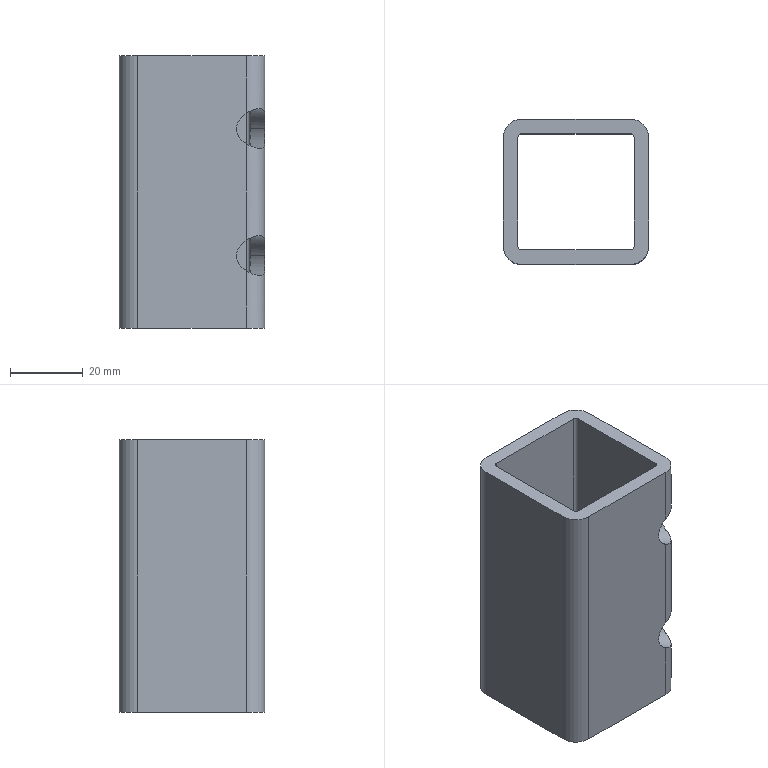Part | SolidWorks | features Extrusion 1, ICE 1 | 1 solid | 26 faces | box 40 x 40 x 75 mm | volume 40690 mm3 | cylinder 16 | plane 10 | commonest cylinder face diameters 2 x6 10 x6 11 x4
STEP:
#1=CARTESIAN_POINT('',(20.,-15.,15.787));
#2=VERTEX_POINT('',#1);
#3=CARTESIAN_POINT('',(20.,-12.222,20.));
#4=VERTEX_POINT('',#3);
#5=CARTESIAN_POINT('',(20.,-15.,15.787));
#6=CARTESIAN_POINT('',(20.,-13.21,16.849));
#7=CARTESIAN_POINT('',(20.,-12.222,18.347));
#8=CARTESIAN_POINT('',(20.,-12.222,20.));
#9=(BOUNDED_CURVE()B_SPLINE_CURVE(3,(#5,#6,#7,#8),.UNSPECIFIED.,.F.,.F.)B_SPLINE_CURVE_WITH_KNOTS((4,4),(5.411,6.283),.UNSPECIFIED.)CURVE()GEOMETRIC_REPRESENTATION_ITEM()RATIONAL_B_SPLINE_CURVE((1.,0.9375,0.9375,1.))REPRESENTATION_ITEM(''));
#10=EDGE_CURVE('',#2,#4,#9,.T.);
#11=ORIENTED_EDGE('',*,*,#10,.T.);
#12=CARTESIAN_POINT('',(16.,-8.222,20.));
#13=VERTEX_POINT('',#12);
#14=CARTESIAN_POINT('',(35.709,-27.931,20.));
#15=DIRECTION('',(-0.7071,0.7071,0.));
#16=VECTOR('',#15,1000.);
#17=LINE('',#14,#16);
#18=EDGE_CURVE('',#4,#13,#17,.T.);
#19=ORIENTED_EDGE('',*,*,#18,.T.);
#20=CARTESIAN_POINT('',(16.,-15.,14.546));
#21=VERTEX_POINT('',#20);
#22=CARTESIAN_POINT('',(16.,-15.,14.546));
#23=CARTESIAN_POINT('',(16.,-10.931,14.919));
#24=CARTESIAN_POINT('',(16.,-8.222,17.098));
#25=CARTESIAN_POINT('',(16.,-8.222,20.));
#26=(BOUNDED_CURVE()B_SPLINE_CURVE(3,(#22,#23,#24,#25),.UNSPECIFIED.,.F.,.F.)B_SPLINE_CURVE_WITH_KNOTS((4,4),(4.841,6.283),.UNSPECIFIED.)CURVE()GEOMETRIC_REPRESENTATION_ITEM()RATIONAL_B_SPLINE_CURVE((1.,0.8341,0.8341,1.))REPRESENTATION_ITEM(''));
#27=EDGE_CURVE('',#21,#13,#26,.T.);
#28=ORIENTED_EDGE('',*,*,#27,.F.);
#29=CARTESIAN_POINT('',(15.,-16.,14.546));
#30=VERTEX_POINT('',#29);
#31=CARTESIAN_POINT('',(16.,-15.,14.546));
#32=CARTESIAN_POINT('',(16.,-15.132,14.534));
#33=CARTESIAN_POINT('',(15.974,-15.261,14.522));
#34=CARTESIAN_POINT('',(15.874,-15.503,14.505));
#35=CARTESIAN_POINT('',(15.8,-15.614,14.5));
#36=CARTESIAN_POINT('',(15.615,-15.799,14.5));
#37=CARTESIAN_POINT('',(15.503,-15.874,14.505));
#38=CARTESIAN_POINT('',(15.263,-15.974,14.522));
#39=CARTESIAN_POINT('',(15.132,-16.,14.534));
#40=CARTESIAN_POINT('',(15.,-16.,14.546));
#41=B_SPLINE_CURVE_WITH_KNOTS('',3,(#31,#32,#33,#34,#35,#36,#37,#38,#39,#40),.UNSPECIFIED.,.F.,.F.,(4,2,2,2,4),(0.,0.0003914,0.0007827,0.001174,0.001565),.UNSPECIFIED.);
#42=EDGE_CURVE('',#21,#30,#41,.T.);
#43=ORIENTED_EDGE('',*,*,#42,.T.);
#44=CARTESIAN_POINT('',(8.222,-16.,20.));
#45=VERTEX_POINT('',#44);
#46=CARTESIAN_POINT('',(15.,-16.,14.546));
#47=CARTESIAN_POINT('',(10.931,-16.,14.919));
#48=CARTESIAN_POINT('',(8.222,-16.,17.098));
#49=CARTESIAN_POINT('',(8.222,-16.,20.));
#50=(BOUNDED_CURVE()B_SPLINE_CURVE(3,(#46,#47,#48,#49),.UNSPECIFIED.,.F.,.F.)B_SPLINE_CURVE_WITH_KNOTS((4,4),(4.841,6.283),.UNSPECIFIED.)CURVE()GEOMETRIC_REPRESENTATION_ITEM()RATIONAL_B_SPLINE_CURVE((1.,0.8341,0.8341,1.))REPRESENTATION_ITEM(''));
#51=EDGE_CURVE('',#30,#45,#50,.T.);
#52=ORIENTED_EDGE('',*,*,#51,.T.);
#53=CARTESIAN_POINT('',(12.222,-20.,20.));
#54=VERTEX_POINT('',#53);
#55=CARTESIAN_POINT('',(27.931,-35.709,20.));
#56=DIRECTION('',(-0.7071,0.7071,0.));
#57=VECTOR('',#56,1000.);
#58=LINE('',#55,#57);
#59=EDGE_CURVE('',#54,#45,#58,.T.);
#60=ORIENTED_EDGE('',*,*,#59,.F.);
#61=CARTESIAN_POINT('',(15.,-20.,15.787));
#62=VERTEX_POINT('',#61);
#63=CARTESIAN_POINT('',(15.,-20.,15.787));
#64=CARTESIAN_POINT('',(13.21,-20.,16.849));
#65=CARTESIAN_POINT('',(12.222,-20.,18.347));
#66=CARTESIAN_POINT('',(12.222,-20.,20.));
#67=(BOUNDED_CURVE()B_SPLINE_CURVE(3,(#63,#64,#65,#66),.UNSPECIFIED.,.F.,.F.)B_SPLINE_CURVE_WITH_KNOTS((4,4),(5.411,6.283),.UNSPECIFIED.)CURVE()GEOMETRIC_REPRESENTATION_ITEM()RATIONAL_B_SPLINE_CURVE((1.,0.9375,0.9375,1.))REPRESENTATION_ITEM(''));
#68=EDGE_CURVE('',#62,#54,#67,.T.);
#69=ORIENTED_EDGE('',*,*,#68,.F.);
#70=CARTESIAN_POINT('',(20.,-15.,15.787));
#71=CARTESIAN_POINT('',(20.,-15.301,15.608));
#72=CARTESIAN_POINT('',(19.973,-15.604,15.44));
#73=CARTESIAN_POINT('',(19.888,-16.063,15.209));
#74=CARTESIAN_POINT('',(19.852,-16.216,15.136));
#75=CARTESIAN_POINT('',(19.764,-16.525,14.997));
#76=CARTESIAN_POINT('',(19.712,-16.68,14.932));
#77=CARTESIAN_POINT('',(19.532,-17.138,14.757));
#78=CARTESIAN_POINT('',(19.38,-17.436,14.664));
#79=CARTESIAN_POINT('',(19.003,-18.016,14.534));
#80=CARTESIAN_POINT('',(18.786,-18.284,14.501));
#81=CARTESIAN_POINT('',(18.419,-18.653,14.5));
#82=CARTESIAN_POINT('',(18.288,-18.771,14.508));
#83=CARTESIAN_POINT('',(18.017,-18.991,14.54));
#84=CARTESIAN_POINT('',(17.878,-19.092,14.565));
#85=CARTESIAN_POINT('',(17.449,-19.373,14.66));
#86=CARTESIAN_POINT('',(17.144,-19.529,14.755));
#87=CARTESIAN_POINT('',(16.534,-19.77,14.988));
#88=CARTESIAN_POINT('',(16.224,-19.858,15.128));
#89=CARTESIAN_POINT('',(15.606,-19.973,15.438));
#90=CARTESIAN_POINT('',(15.302,-20.,15.608));
#91=CARTESIAN_POINT('',(15.,-20.,15.787));
#92=B_SPLINE_CURVE_WITH_KNOTS('',3,(#70,#71,#72,#73,#74,#75,#76,#77,#78,#79,#80,#81,#82,#83,#84,#85,#86,#87,#88,#89,#90,#91),.UNSPECIFIED.,.F.,.F.,(4,2,2,2,2,2,2,2,2,2,4),(0.,0.00104,0.00156,0.00208,0.00312,0.00416,0.00468,0.0052,0.00624,0.00728,0.00832),.UNSPECIFIED.);
#93=EDGE_CURVE('',#2,#62,#92,.T.);
#94=ORIENTED_EDGE('',*,*,#93,.F.);
#95=EDGE_LOOP('',(#11,#19,#28,#43,#52,#60,#69,#94));
#96=FACE_OUTER_BOUND('',#95,.T.);
#97=CARTESIAN_POINT('',(31.82,-31.82,20.));
#98=DIRECTION('',(-0.7071,0.7071,0.));
#99=DIRECTION('',(-0.7071,-0.7071,0.));
#100=AXIS2_PLACEMENT_3D('',#97,#98,#99);
#101=CYLINDRICAL_SURFACE('',#100,5.5);
#102=ADVANCED_FACE('',(#96),#101,.F.);
#103=CARTESIAN_POINT('',(20.,-15.,50.787));
#104=VERTEX_POINT('',#103);
#105=CARTESIAN_POINT('',(20.,-12.222,55.));
#106=VERTEX_POINT('',#105);
#107=CARTESIAN_POINT('',(20.,-15.,50.787));
#108=CARTESIAN_POINT('',(20.,-13.21,51.849));
#109=CARTESIAN_POINT('',(20.,-12.222,53.347));
#110=CARTESIAN_POINT('',(20.,-12.222,55.));
#111=(BOUNDED_CURVE()B_SPLINE_CURVE(3,(#107,#108,#109,#110),.UNSPECIFIED.,.F.,.F.)B_SPLINE_CURVE_WITH_KNOTS((4,4),(5.411,6.283),.UNSPECIFIED.)CURVE()GEOMETRIC_REPRESENTATION_ITEM()RATIONAL_B_SPLINE_CURVE((1.,0.9375,0.9375,1.))REPRESENTATION_ITEM(''));
#112=EDGE_CURVE('',#104,#106,#111,.T.);
#113=ORIENTED_EDGE('',*,*,#112,.T.);
#114=CARTESIAN_POINT('',(16.,-8.222,55.));
#115=VERTEX_POINT('',#114);
#116=CARTESIAN_POINT('',(35.709,-27.931,55.));
#117=DIRECTION('',(-0.7071,0.7071,0.));
#118=VECTOR('',#117,1000.);
#119=LINE('',#116,#118);
#120=EDGE_CURVE('',#106,#115,#119,.T.);
#121=ORIENTED_EDGE('',*,*,#120,.T.);
#122=CARTESIAN_POINT('',(16.,-15.,49.546));
#123=VERTEX_POINT('',#122);
#124=CARTESIAN_POINT('',(16.,-15.,49.546));
#125=CARTESIAN_POINT('',(16.,-10.931,49.919));
#126=CARTESIAN_POINT('',(16.,-8.222,52.098));
#127=CARTESIAN_POINT('',(16.,-8.222,55.));
#128=(BOUNDED_CURVE()B_SPLINE_CURVE(3,(#124,#125,#126,#127),.UNSPECIFIED.,.F.,.F.)B_SPLINE_CURVE_WITH_KNOTS((4,4),(4.841,6.283),.UNSPECIFIED.)CURVE()GEOMETRIC_REPRESENTATION_ITEM()RATIONAL_B_SPLINE_CURVE((1.,0.8341,0.8341,1.))REPRESENTATION_ITEM(''));
#129=EDGE_CURVE('',#123,#115,#128,.T.);
#130=ORIENTED_EDGE('',*,*,#129,.F.);
#131=CARTESIAN_POINT('',(15.,-16.,49.546));
#132=VERTEX_POINT('',#131);
#133=CARTESIAN_POINT('',(16.,-15.,49.546));
#134=CARTESIAN_POINT('',(16.,-15.132,49.534));
#135=CARTESIAN_POINT('',(15.974,-15.261,49.522));
#136=CARTESIAN_POINT('',(15.874,-15.503,49.505));
#137=CARTESIAN_POINT('',(15.8,-15.614,49.5));
#138=CARTESIAN_POINT('',(15.615,-15.799,49.5));
#139=CARTESIAN_POINT('',(15.503,-15.874,49.505));
#140=CARTESIAN_POINT('',(15.263,-15.974,49.522));
#141=CARTESIAN_POINT('',(15.132,-16.,49.534));
#142=CARTESIAN_POINT('',(15.,-16.,49.546));
#143=B_SPLINE_CURVE_WITH_KNOTS('',3,(#133,#134,#135,#136,#137,#138,#139,#140,#141,#142),.UNSPECIFIED.,.F.,.F.,(4,2,2,2,4),(0.,0.0003914,0.0007827,0.001174,0.001565),.UNSPECIFIED.);
#144=EDGE_CURVE('',#123,#132,#143,.T.);
#145=ORIENTED_EDGE('',*,*,#144,.T.);
#146=CARTESIAN_POINT('',(8.222,-16.,55.));
#147=VERTEX_POINT('',#146);
#148=CARTESIAN_POINT('',(15.,-16.,49.546));
#149=CARTESIAN_POINT('',(10.931,-16.,49.919));
#150=CARTESIAN_POINT('',(8.222,-16.,52.098));
#151=CARTESIAN_POINT('',(8.222,-16.,55.));
#152=(BOUNDED_CURVE()B_SPLINE_CURVE(3,(#148,#149,#150,#151),.UNSPECIFIED.,.F.,.F.)B_SPLINE_CURVE_WITH_KNOTS((4,4),(4.841,6.283),.UNSPECIFIED.)CURVE()GEOMETRIC_REPRESENTATION_ITEM()RATIONAL_B_SPLINE_CURVE((1.,0.8341,0.8341,1.))REPRESENTATION_ITEM(''));
#153=EDGE_CURVE('',#132,#147,#152,.T.);
#154=ORIENTED_EDGE('',*,*,#153,.T.);
#155=CARTESIAN_POINT('',(12.222,-20.,55.));
#156=VERTEX_POINT('',#155);
#157=CARTESIAN_POINT('',(27.931,-35.709,55.));
#158=DIRECTION('',(-0.7071,0.7071,0.));
#159=VECTOR('',#158,1000.);
#160=LINE('',#157,#159);
#161=EDGE_CURVE('',#156,#147,#160,.T.);
#162=ORIENTED_EDGE('',*,*,#161,.F.);
#163=CARTESIAN_POINT('',(15.,-20.,50.787));
#164=VERTEX_POINT('',#163);
#165=CARTESIAN_POINT('',(15.,-20.,50.787));
#166=CARTESIAN_POINT('',(13.21,-20.,51.849));
#167=CARTESIAN_POINT('',(12.222,-20.,53.347));
#168=CARTESIAN_POINT('',(12.222,-20.,55.));
#169=(BOUNDED_CURVE()B_SPLINE_CURVE(3,(#165,#166,#167,#168),.UNSPECIFIED.,.F.,.F.)B_SPLINE_CURVE_WITH_KNOTS((4,4),(5.411,6.283),.UNSPECIFIED.)CURVE()GEOMETRIC_REPRESENTATION_ITEM()RATIONAL_B_SPLINE_CURVE((1.,0.9375,0.9375,1.))REPRESENTATION_ITEM(''));
#170=EDGE_CURVE('',#164,#156,#169,.T.);
#171=ORIENTED_EDGE('',*,*,#170,.F.);
#172=CARTESIAN_POINT('',(20.,-15.,50.787));
#173=CARTESIAN_POINT('',(20.,-15.301,50.608));
#174=CARTESIAN_POINT('',(19.973,-15.604,50.44));
#175=CARTESIAN_POINT('',(19.888,-16.063,50.209));
#176=CARTESIAN_POINT('',(19.852,-16.216,50.136));
#177=CARTESIAN_POINT('',(19.764,-16.525,49.997));
#178=CARTESIAN_POINT('',(19.712,-16.68,49.932));
#179=CARTESIAN_POINT('',(19.532,-17.138,49.757));
#180=CARTESIAN_POINT('',(19.38,-17.436,49.664));
#181=CARTESIAN_POINT('',(19.003,-18.016,49.534));
#182=CARTESIAN_POINT('',(18.786,-18.284,49.501));
#183=CARTESIAN_POINT('',(18.419,-18.653,49.5));
#184=CARTESIAN_POINT('',(18.288,-18.771,49.508));
#185=CARTESIAN_POINT('',(18.017,-18.991,49.54));
#186=CARTESIAN_POINT('',(17.878,-19.092,49.565));
#187=CARTESIAN_POINT('',(17.449,-19.373,49.66));
#188=CARTESIAN_POINT('',(17.144,-19.529,49.755));
#189=CARTESIAN_POINT('',(16.534,-19.77,49.988));
#190=CARTESIAN_POINT('',(16.224,-19.858,50.128));
#191=CARTESIAN_POINT('',(15.606,-19.973,50.438));
#192=CARTESIAN_POINT('',(15.302,-20.,50.608));
#193=CARTESIAN_POINT('',(15.,-20.,50.787));
#194=B_SPLINE_CURVE_WITH_KNOTS('',3,(#172,#173,#174,#175,#176,#177,#178,#179,#180,#181,#182,#183,#184,#185,#186,#187,#188,#189,#190,#191,#192,#193),.UNSPECIFIED.,.F.,.F.,(4,2,2,2,2,2,2,2,2,2,4),(0.,0.00104,0.00156,0.00208,0.00312,0.00416,0.00468,0.0052,0.00624,0.00728,0.00832),.UNSPECIFIED.);
#195=EDGE_CURVE('',#104,#164,#194,.T.);
#196=ORIENTED_EDGE('',*,*,#195,.F.);
#197=EDGE_LOOP('',(#113,#121,#130,#145,#154,#162,#171,#196));
#198=FACE_OUTER_BOUND('',#197,.T.);
#199=CARTESIAN_POINT('',(31.82,-31.82,55.));
#200=DIRECTION('',(-0.7071,0.7071,0.));
#201=DIRECTION('',(-0.7071,-0.7071,0.));
#202=AXIS2_PLACEMENT_3D('',#199,#200,#201);
#203=CYLINDRICAL_SURFACE('',#202,5.5);
#204=ADVANCED_FACE('',(#198),#203,.F.);
#205=CARTESIAN_POINT('',(15.,-20.,24.213));
#206=VERTEX_POINT('',#205);
#207=CARTESIAN_POINT('',(15.,-20.,75.));
#208=DIRECTION('',(0.,0.,-1.));
#209=VECTOR('',#208,1000.);
#210=LINE('',#207,#209);
#211=EDGE_CURVE('',#164,#206,#210,.T.);
#212=ORIENTED_EDGE('',*,*,#211,.T.);
#213=CARTESIAN_POINT('',(20.,-15.,24.213));
#214=VERTEX_POINT('',#213);
#215=CARTESIAN_POINT('',(15.,-20.,24.213));
#216=CARTESIAN_POINT('',(15.301,-20.,24.392));
#217=CARTESIAN_POINT('',(15.604,-19.973,24.56));
#218=CARTESIAN_POINT('',(16.063,-19.888,24.791));
#219=CARTESIAN_POINT('',(16.216,-19.852,24.864));
#220=CARTESIAN_POINT('',(16.525,-19.764,25.003));
#221=CARTESIAN_POINT('',(16.68,-19.712,25.068));
#222=CARTESIAN_POINT('',(17.138,-19.532,25.243));
#223=CARTESIAN_POINT('',(17.436,-19.38,25.336));
#224=CARTESIAN_POINT('',(18.016,-19.003,25.466));
#225=CARTESIAN_POINT('',(18.284,-18.786,25.499));
#226=CARTESIAN_POINT('',(18.653,-18.419,25.5));
#227=CARTESIAN_POINT('',(18.771,-18.288,25.492));
#228=CARTESIAN_POINT('',(18.991,-18.017,25.46));
#229=CARTESIAN_POINT('',(19.092,-17.878,25.435));
#230=CARTESIAN_POINT('',(19.373,-17.449,25.34));
#231=CARTESIAN_POINT('',(19.529,-17.144,25.245));
#232=CARTESIAN_POINT('',(19.77,-16.534,25.012));
#233=CARTESIAN_POINT('',(19.858,-16.224,24.872));
#234=CARTESIAN_POINT('',(19.973,-15.606,24.562));
#235=CARTESIAN_POINT('',(20.,-15.302,24.392));
#236=CARTESIAN_POINT('',(20.,-15.,24.213));
#237=B_SPLINE_CURVE_WITH_KNOTS('',3,(#215,#216,#217,#218,#219,#220,#221,#222,#223,#224,#225,#226,#227,#228,#229,#230,#231,#232,#233,#234,#235,#236),.UNSPECIFIED.,.F.,.F.,(4,2,2,2,2,2,2,2,2,2,4),(0.,0.00104,0.00156,0.00208,0.00312,0.00416,0.00468,0.0052,0.00624,0.00728,0.00832),.UNSPECIFIED.);
#238=EDGE_CURVE('',#206,#214,#237,.T.);
#239=ORIENTED_EDGE('',*,*,#238,.T.);
#240=CARTESIAN_POINT('',(20.,-15.,75.));
#241=DIRECTION('',(0.,0.,-1.));
#242=VECTOR('',#241,1000.);
#243=LINE('',#240,#242);
#244=EDGE_CURVE('',#104,#214,#243,.T.);
#245=ORIENTED_EDGE('',*,*,#244,.F.);
#246=ORIENTED_EDGE('',*,*,#195,.T.);
#247=EDGE_LOOP('',(#212,#239,#245,#246));
#248=FACE_OUTER_BOUND('',#247,.T.);
#249=CARTESIAN_POINT('',(15.,-15.,75.));
#250=DIRECTION('',(0.,0.,-1.));
#251=DIRECTION('',(-1.,0.,0.));
#252=AXIS2_PLACEMENT_3D('',#249,#250,#251);
#253=CYLINDRICAL_SURFACE('',#252,5.);
#254=ADVANCED_FACE('',(#248),#253,.T.);
#255=CARTESIAN_POINT('',(15.,-20.,75.));
#256=VERTEX_POINT('',#255);
#257=CARTESIAN_POINT('',(15.,-20.,59.213));
#258=VERTEX_POINT('',#257);
#259=CARTESIAN_POINT('',(15.,-20.,75.));
#260=DIRECTION('',(0.,0.,-1.));
#261=VECTOR('',#260,1000.);
#262=LINE('',#259,#261);
#263=EDGE_CURVE('',#256,#258,#262,.T.);
#264=ORIENTED_EDGE('',*,*,#263,.T.);
#265=CARTESIAN_POINT('',(20.,-15.,59.213));
#266=VERTEX_POINT('',#265);
#267=CARTESIAN_POINT('',(15.,-20.,59.213));
#268=CARTESIAN_POINT('',(15.301,-20.,59.392));
#269=CARTESIAN_POINT('',(15.604,-19.973,59.56));
#270=CARTESIAN_POINT('',(16.063,-19.888,59.791));
#271=CARTESIAN_POINT('',(16.216,-19.852,59.864));
#272=CARTESIAN_POINT('',(16.525,-19.764,60.003));
#273=CARTESIAN_POINT('',(16.68,-19.712,60.068));
#274=CARTESIAN_POINT('',(17.138,-19.532,60.243));
#275=CARTESIAN_POINT('',(17.436,-19.38,60.336));
#276=CARTESIAN_POINT('',(18.016,-19.003,60.466));
#277=CARTESIAN_POINT('',(18.284,-18.786,60.499));
#278=CARTESIAN_POINT('',(18.653,-18.419,60.5));
#279=CARTESIAN_POINT('',(18.771,-18.288,60.492));
#280=CARTESIAN_POINT('',(18.991,-18.017,60.46));
#281=CARTESIAN_POINT('',(19.092,-17.878,60.435));
#282=CARTESIAN_POINT('',(19.373,-17.449,60.34));
#283=CARTESIAN_POINT('',(19.529,-17.144,60.245));
#284=CARTESIAN_POINT('',(19.77,-16.534,60.012));
#285=CARTESIAN_POINT('',(19.858,-16.224,59.872));
#286=CARTESIAN_POINT('',(19.973,-15.606,59.562));
#287=CARTESIAN_POINT('',(20.,-15.302,59.392));
#288=CARTESIAN_POINT('',(20.,-15.,59.213));
#289=B_SPLINE_CURVE_WITH_KNOTS('',3,(#267,#268,#269,#270,#271,#272,#273,#274,#275,#276,#277,#278,#279,#280,#281,#282,#283,#284,#285,#286,#287,#288),.UNSPECIFIED.,.F.,.F.,(4,2,2,2,2,2,2,2,2,2,4),(0.,0.00104,0.00156,0.00208,0.00312,0.00416,0.00468,0.0052,0.00624,0.00728,0.00832),.UNSPECIFIED.);
#290=EDGE_CURVE('',#258,#266,#289,.T.);
#291=ORIENTED_EDGE('',*,*,#290,.T.);
#292=CARTESIAN_POINT('',(20.,-15.,75.));
#293=VERTEX_POINT('',#292);
#294=CARTESIAN_POINT('',(20.,-15.,75.));
#295=DIRECTION('',(0.,0.,-1.));
#296=VECTOR('',#295,1000.);
#297=LINE('',#294,#296);
#298=EDGE_CURVE('',#293,#266,#297,.T.);
#299=ORIENTED_EDGE('',*,*,#298,.F.);
#300=CARTESIAN_POINT('',(15.,-15.,75.));
#301=DIRECTION('',(0.,0.,1.));
#302=DIRECTION('',(1.,0.,0.));
#303=AXIS2_PLACEMENT_3D('',#300,#301,#302);
#304=CIRCLE('',#303,5.);
#305=EDGE_CURVE('',#256,#293,#304,.T.);
#306=ORIENTED_EDGE('',*,*,#305,.F.);
#307=EDGE_LOOP('',(#264,#291,#299,#306));
#308=FACE_OUTER_BOUND('',#307,.T.);
#309=CARTESIAN_POINT('',(15.,-15.,75.));
#310=DIRECTION('',(0.,0.,-1.));
#311=DIRECTION('',(-1.,0.,0.));
#312=AXIS2_PLACEMENT_3D('',#309,#310,#311);
#313=CYLINDRICAL_SURFACE('',#312,5.);
#314=ADVANCED_FACE('',(#308),#313,.T.);
#315=CARTESIAN_POINT('',(15.,-16.,25.454));
#316=VERTEX_POINT('',#315);
#317=CARTESIAN_POINT('',(16.,-15.,25.454));
#318=VERTEX_POINT('',#317);
#319=CARTESIAN_POINT('',(15.,-16.,25.454));
#320=CARTESIAN_POINT('',(15.132,-16.,25.466));
#321=CARTESIAN_POINT('',(15.261,-15.974,25.478));
#322=CARTESIAN_POINT('',(15.503,-15.874,25.495));
#323=CARTESIAN_POINT('',(15.614,-15.8,25.5));
#324=CARTESIAN_POINT('',(15.799,-15.615,25.5));
#325=CARTESIAN_POINT('',(15.874,-15.503,25.495));
#326=CARTESIAN_POINT('',(15.974,-15.263,25.478));
#327=CARTESIAN_POINT('',(16.,-15.132,25.466));
#328=CARTESIAN_POINT('',(16.,-15.,25.454));
#329=B_SPLINE_CURVE_WITH_KNOTS('',3,(#319,#320,#321,#322,#323,#324,#325,#326,#327,#328),.UNSPECIFIED.,.F.,.F.,(4,2,2,2,4),(0.,0.0003914,0.0007827,0.001174,0.001565),.UNSPECIFIED.);
#330=EDGE_CURVE('',#316,#318,#329,.T.);
#331=ORIENTED_EDGE('',*,*,#330,.F.);
#332=CARTESIAN_POINT('',(15.,-16.,75.));
#333=DIRECTION('',(0.,0.,-1.));
#334=VECTOR('',#333,1000.);
#335=LINE('',#332,#334);
#336=EDGE_CURVE('',#132,#316,#335,.T.);
#337=ORIENTED_EDGE('',*,*,#336,.F.);
#338=ORIENTED_EDGE('',*,*,#144,.F.);
#339=CARTESIAN_POINT('',(16.,-15.,75.));
#340=DIRECTION('',(0.,0.,-1.));
#341=VECTOR('',#340,1000.);
#342=LINE('',#339,#341);
#343=EDGE_CURVE('',#123,#318,#342,.T.);
#344=ORIENTED_EDGE('',*,*,#343,.T.);
#345=EDGE_LOOP('',(#331,#337,#338,#344));
#346=FACE_OUTER_BOUND('',#345,.T.);
#347=CARTESIAN_POINT('',(15.,-15.,75.));
#348=DIRECTION('',(0.,0.,-1.));
#349=DIRECTION('',(-1.,0.,0.));
#350=AXIS2_PLACEMENT_3D('',#347,#348,#349);
#351=CYLINDRICAL_SURFACE('',#350,1.);
#352=ADVANCED_FACE('',(#346),#351,.F.);
#353=CARTESIAN_POINT('',(15.,-16.,60.454));
#354=VERTEX_POINT('',#353);
#355=CARTESIAN_POINT('',(16.,-15.,60.454));
#356=VERTEX_POINT('',#355);
#357=CARTESIAN_POINT('',(15.,-16.,60.454));
#358=CARTESIAN_POINT('',(15.132,-16.,60.466));
#359=CARTESIAN_POINT('',(15.261,-15.974,60.478));
#360=CARTESIAN_POINT('',(15.503,-15.874,60.495));
#361=CARTESIAN_POINT('',(15.614,-15.8,60.5));
#362=CARTESIAN_POINT('',(15.799,-15.615,60.5));
#363=CARTESIAN_POINT('',(15.874,-15.503,60.495));
#364=CARTESIAN_POINT('',(15.974,-15.263,60.478));
#365=CARTESIAN_POINT('',(16.,-15.132,60.466));
#366=CARTESIAN_POINT('',(16.,-15.,60.454));
#367=B_SPLINE_CURVE_WITH_KNOTS('',3,(#357,#358,#359,#360,#361,#362,#363,#364,#365,#366),.UNSPECIFIED.,.F.,.F.,(4,2,2,2,4),(0.,0.0003914,0.0007827,0.001174,0.001565),.UNSPECIFIED.);
#368=EDGE_CURVE('',#354,#356,#367,.T.);
#369=ORIENTED_EDGE('',*,*,#368,.F.);
#370=CARTESIAN_POINT('',(15.,-16.,75.));
#371=VERTEX_POINT('',#370);
#372=CARTESIAN_POINT('',(15.,-16.,75.));
#373=DIRECTION('',(0.,0.,-1.));
#374=VECTOR('',#373,1000.);
#375=LINE('',#372,#374);
#376=EDGE_CURVE('',#371,#354,#375,.T.);
#377=ORIENTED_EDGE('',*,*,#376,.F.);
#378=CARTESIAN_POINT('',(16.,-15.,75.));
#379=VERTEX_POINT('',#378);
#380=CARTESIAN_POINT('',(15.,-15.,75.));
#381=DIRECTION('',(0.,0.,1.));
#382=DIRECTION('',(1.,0.,0.));
#383=AXIS2_PLACEMENT_3D('',#380,#381,#382);
#384=CIRCLE('',#383,1.);
#385=EDGE_CURVE('',#371,#379,#384,.T.);
#386=ORIENTED_EDGE('',*,*,#385,.T.);
#387=CARTESIAN_POINT('',(16.,-15.,75.));
#388=DIRECTION('',(0.,0.,-1.));
#389=VECTOR('',#388,1000.);
#390=LINE('',#387,#389);
#391=EDGE_CURVE('',#379,#356,#390,.T.);
#392=ORIENTED_EDGE('',*,*,#391,.T.);
#393=EDGE_LOOP('',(#369,#377,#386,#392));
#394=FACE_OUTER_BOUND('',#393,.T.);
#395=CARTESIAN_POINT('',(15.,-15.,75.));
#396=DIRECTION('',(0.,0.,-1.));
#397=DIRECTION('',(-1.,0.,0.));
#398=AXIS2_PLACEMENT_3D('',#395,#396,#397);
#399=CYLINDRICAL_SURFACE('',#398,1.);
#400=ADVANCED_FACE('',(#394),#399,.F.);
#401=CARTESIAN_POINT('',(-15.,20.,0.));
#402=VERTEX_POINT('',#401);
#403=CARTESIAN_POINT('',(-20.,15.,0.));
#404=VERTEX_POINT('',#403);
#405=CARTESIAN_POINT('',(-15.,15.,0.));
#406=DIRECTION('',(0.,0.,1.));
#407=DIRECTION('',(1.,0.,0.));
#408=AXIS2_PLACEMENT_3D('',#405,#406,#407);
#409=CIRCLE('',#408,5.);
#410=EDGE_CURVE('',#402,#404,#409,.T.);
#411=ORIENTED_EDGE('',*,*,#410,.T.);
#412=CARTESIAN_POINT('',(-20.,15.,75.));
#413=VERTEX_POINT('',#412);
#414=CARTESIAN_POINT('',(-20.,15.,75.));
#415=DIRECTION('',(0.,0.,-1.));
#416=VECTOR('',#415,1000.);
#417=LINE('',#414,#416);
#418=EDGE_CURVE('',#413,#404,#417,.T.);
#419=ORIENTED_EDGE('',*,*,#418,.F.);
#420=CARTESIAN_POINT('',(-15.,20.,75.));
#421=VERTEX_POINT('',#420);
#422=CARTESIAN_POINT('',(-15.,15.,75.));
#423=DIRECTION('',(0.,0.,1.));
#424=DIRECTION('',(1.,0.,0.));
#425=AXIS2_PLACEMENT_3D('',#422,#423,#424);
#426=CIRCLE('',#425,5.);
#427=EDGE_CURVE('',#421,#413,#426,.T.);
#428=ORIENTED_EDGE('',*,*,#427,.F.);
#429=CARTESIAN_POINT('',(-15.,20.,75.));
#430=DIRECTION('',(0.,0.,-1.));
#431=VECTOR('',#430,1000.);
#432=LINE('',#429,#431);
#433=EDGE_CURVE('',#421,#402,#432,.T.);
#434=ORIENTED_EDGE('',*,*,#433,.T.);
#435=EDGE_LOOP('',(#411,#419,#428,#434));
#436=FACE_OUTER_BOUND('',#435,.T.);
#437=CARTESIAN_POINT('',(-15.,15.,75.));
#438=DIRECTION('',(0.,0.,-1.));
#439=DIRECTION('',(-1.,0.,0.));
#440=AXIS2_PLACEMENT_3D('',#437,#438,#439);
#441=CYLINDRICAL_SURFACE('',#440,5.);
#442=ADVANCED_FACE('',(#436),#441,.T.);
#443=CARTESIAN_POINT('',(-20.,-15.,0.));
#444=VERTEX_POINT('',#443);
#445=CARTESIAN_POINT('',(-20.,15.,0.));
#446=DIRECTION('',(0.,-1.,0.));
#447=VECTOR('',#446,1000.);
#448=LINE('',#445,#447);
#449=EDGE_CURVE('',#404,#444,#448,.T.);
#450=ORIENTED_EDGE('',*,*,#449,.T.);
#451=CARTESIAN_POINT('',(-20.,-15.,75.));
#452=VERTEX_POINT('',#451);
#453=CARTESIAN_POINT('',(-20.,-15.,75.));
#454=DIRECTION('',(0.,0.,-1.));
#455=VECTOR('',#454,1000.);
#456=LINE('',#453,#455);
#457=EDGE_CURVE('',#452,#444,#456,.T.);
#458=ORIENTED_EDGE('',*,*,#457,.F.);
#459=CARTESIAN_POINT('',(-20.,15.,75.));
#460=DIRECTION('',(0.,-1.,0.));
#461=VECTOR('',#460,1000.);
#462=LINE('',#459,#461);
#463=EDGE_CURVE('',#413,#452,#462,.T.);
#464=ORIENTED_EDGE('',*,*,#463,.F.);
#465=ORIENTED_EDGE('',*,*,#418,.T.);
#466=EDGE_LOOP('',(#450,#458,#464,#465));
#467=FACE_OUTER_BOUND('',#466,.T.);
#468=CARTESIAN_POINT('',(-20.,15.,75.));
#469=DIRECTION('',(1.,0.,0.));
#470=DIRECTION('',(0.,0.,-1.));
#471=AXIS2_PLACEMENT_3D('',#468,#469,#470);
#472=PLANE('',#471);
#473=ADVANCED_FACE('',(#467),#472,.F.);
#474=CARTESIAN_POINT('',(-15.,-20.,0.));
#475=VERTEX_POINT('',#474);
#476=CARTESIAN_POINT('',(-15.,-15.,0.));
#477=DIRECTION('',(0.,0.,1.));
#478=DIRECTION('',(1.,0.,0.));
#479=AXIS2_PLACEMENT_3D('',#476,#477,#478);
#480=CIRCLE('',#479,5.);
#481=EDGE_CURVE('',#444,#475,#480,.T.);
#482=ORIENTED_EDGE('',*,*,#481,.T.);
#483=CARTESIAN_POINT('',(-15.,-20.,75.));
#484=VERTEX_POINT('',#483);
#485=CARTESIAN_POINT('',(-15.,-20.,75.));
#486=DIRECTION('',(0.,0.,-1.));
#487=VECTOR('',#486,1000.);
#488=LINE('',#485,#487);
#489=EDGE_CURVE('',#484,#475,#488,.T.);
#490=ORIENTED_EDGE('',*,*,#489,.F.);
#491=CARTESIAN_POINT('',(-15.,-15.,75.));
#492=DIRECTION('',(0.,0.,1.));
#493=DIRECTION('',(1.,0.,0.));
#494=AXIS2_PLACEMENT_3D('',#491,#492,#493);
#495=CIRCLE('',#494,5.);
#496=EDGE_CURVE('',#452,#484,#495,.T.);
#497=ORIENTED_EDGE('',*,*,#496,.F.);
#498=ORIENTED_EDGE('',*,*,#457,.T.);
#499=EDGE_LOOP('',(#482,#490,#497,#498));
#500=FACE_OUTER_BOUND('',#499,.T.);
#501=CARTESIAN_POINT('',(-15.,-15.,75.));
#502=DIRECTION('',(0.,0.,-1.));
#503=DIRECTION('',(-1.,0.,0.));
#504=AXIS2_PLACEMENT_3D('',#501,#502,#503);
#505=CYLINDRICAL_SURFACE('',#504,5.);
#506=ADVANCED_FACE('',(#500),#505,.T.);
#507=CARTESIAN_POINT('',(15.,-20.,0.));
#508=VERTEX_POINT('',#507);
#509=CARTESIAN_POINT('',(15.,-20.,75.));
#510=DIRECTION('',(0.,0.,-1.));
#511=VECTOR('',#510,1000.);
#512=LINE('',#509,#511);
#513=EDGE_CURVE('',#62,#508,#512,.T.);
#514=ORIENTED_EDGE('',*,*,#513,.F.);
#515=ORIENTED_EDGE('',*,*,#68,.T.);
#516=CARTESIAN_POINT('',(12.222,-20.,20.));
#517=CARTESIAN_POINT('',(12.222,-20.,21.653));
#518=CARTESIAN_POINT('',(13.21,-20.,23.151));
#519=CARTESIAN_POINT('',(15.,-20.,24.213));
#520=(BOUNDED_CURVE()B_SPLINE_CURVE(3,(#516,#517,#518,#519),.UNSPECIFIED.,.F.,.F.)B_SPLINE_CURVE_WITH_KNOTS((4,4),(0.,0.8726),.UNSPECIFIED.)CURVE()GEOMETRIC_REPRESENTATION_ITEM()RATIONAL_B_SPLINE_CURVE((1.,0.9375,0.9375,1.))REPRESENTATION_ITEM(''));
#521=EDGE_CURVE('',#54,#206,#520,.T.);
#522=ORIENTED_EDGE('',*,*,#521,.T.);
#523=ORIENTED_EDGE('',*,*,#211,.F.);
#524=ORIENTED_EDGE('',*,*,#170,.T.);
#525=CARTESIAN_POINT('',(12.222,-20.,55.));
#526=CARTESIAN_POINT('',(12.222,-20.,56.653));
#527=CARTESIAN_POINT('',(13.21,-20.,58.151));
#528=CARTESIAN_POINT('',(15.,-20.,59.213));
#529=(BOUNDED_CURVE()B_SPLINE_CURVE(3,(#525,#526,#527,#528),.UNSPECIFIED.,.F.,.F.)B_SPLINE_CURVE_WITH_KNOTS((4,4),(0.,0.8726),.UNSPECIFIED.)CURVE()GEOMETRIC_REPRESENTATION_ITEM()RATIONAL_B_SPLINE_CURVE((1.,0.9375,0.9375,1.))REPRESENTATION_ITEM(''));
#530=EDGE_CURVE('',#156,#258,#529,.T.);
#531=ORIENTED_EDGE('',*,*,#530,.T.);
#532=ORIENTED_EDGE('',*,*,#263,.F.);
#533=CARTESIAN_POINT('',(-15.,-20.,75.));
#534=DIRECTION('',(1.,0.,0.));
#535=VECTOR('',#534,1000.);
#536=LINE('',#533,#535);
#537=EDGE_CURVE('',#484,#256,#536,.T.);
#538=ORIENTED_EDGE('',*,*,#537,.F.);
#539=ORIENTED_EDGE('',*,*,#489,.T.);
#540=CARTESIAN_POINT('',(-15.,-20.,0.));
#541=DIRECTION('',(1.,0.,0.));
#542=VECTOR('',#541,1000.);
#543=LINE('',#540,#542);
#544=EDGE_CURVE('',#475,#508,#543,.T.);
#545=ORIENTED_EDGE('',*,*,#544,.T.);
#546=EDGE_LOOP('',(#514,#515,#522,#523,#524,#531,#532,#538,#539,#545));
#547=FACE_OUTER_BOUND('',#546,.T.);
#548=CARTESIAN_POINT('',(-15.,-20.,75.));
#549=DIRECTION('',(0.,1.,0.));
#550=DIRECTION('',(0.,0.,1.));
#551=AXIS2_PLACEMENT_3D('',#548,#549,#550);
#552=PLANE('',#551);
#553=ADVANCED_FACE('',(#547),#552,.F.);
#554=CARTESIAN_POINT('',(20.,-15.,0.));
#555=VERTEX_POINT('',#554);
#556=CARTESIAN_POINT('',(20.,-15.,75.));
#557=DIRECTION('',(0.,0.,-1.));
#558=VECTOR('',#557,1000.);
#559=LINE('',#556,#558);
#560=EDGE_CURVE('',#2,#555,#559,.T.);
#561=ORIENTED_EDGE('',*,*,#560,.F.);
#562=ORIENTED_EDGE('',*,*,#93,.T.);
#563=ORIENTED_EDGE('',*,*,#513,.T.);
#564=CARTESIAN_POINT('',(15.,-15.,0.));
#565=DIRECTION('',(0.,0.,1.));
#566=DIRECTION('',(1.,0.,0.));
#567=AXIS2_PLACEMENT_3D('',#564,#565,#566);
#568=CIRCLE('',#567,5.);
#569=EDGE_CURVE('',#508,#555,#568,.T.);
#570=ORIENTED_EDGE('',*,*,#569,.T.);
#571=EDGE_LOOP('',(#561,#562,#563,#570));
#572=FACE_OUTER_BOUND('',#571,.T.);
#573=CARTESIAN_POINT('',(15.,-15.,75.));
#574=DIRECTION('',(0.,0.,-1.));
#575=DIRECTION('',(-1.,0.,0.));
#576=AXIS2_PLACEMENT_3D('',#573,#574,#575);
#577=CYLINDRICAL_SURFACE('',#576,5.);
#578=ADVANCED_FACE('',(#572),#577,.T.);
#579=ORIENTED_EDGE('',*,*,#10,.F.);
#580=ORIENTED_EDGE('',*,*,#560,.T.);
#581=CARTESIAN_POINT('',(20.,15.,0.));
#582=VERTEX_POINT('',#581);
#583=CARTESIAN_POINT('',(20.,15.,0.));
#584=DIRECTION('',(0.,-1.,0.));
#585=VECTOR('',#584,1000.);
#586=LINE('',#583,#585);
#587=EDGE_CURVE('',#582,#555,#586,.T.);
#588=ORIENTED_EDGE('',*,*,#587,.F.);
#589=CARTESIAN_POINT('',(20.,15.,75.));
#590=VERTEX_POINT('',#589);
#591=CARTESIAN_POINT('',(20.,15.,75.));
#592=DIRECTION('',(0.,0.,-1.));
#593=VECTOR('',#592,1000.);
#594=LINE('',#591,#593);
#595=EDGE_CURVE('',#590,#582,#594,.T.);
#596=ORIENTED_EDGE('',*,*,#595,.F.);
#597=CARTESIAN_POINT('',(20.,15.,75.));
#598=DIRECTION('',(0.,-1.,0.));
#599=VECTOR('',#598,1000.);
#600=LINE('',#597,#599);
#601=EDGE_CURVE('',#590,#293,#600,.T.);
#602=ORIENTED_EDGE('',*,*,#601,.T.);
#603=ORIENTED_EDGE('',*,*,#298,.T.);
#604=CARTESIAN_POINT('',(20.,-12.222,55.));
#605=CARTESIAN_POINT('',(20.,-12.222,56.653));
#606=CARTESIAN_POINT('',(20.,-13.21,58.151));
#607=CARTESIAN_POINT('',(20.,-15.,59.213));
#608=(BOUNDED_CURVE()B_SPLINE_CURVE(3,(#604,#605,#606,#607),.UNSPECIFIED.,.F.,.F.)B_SPLINE_CURVE_WITH_KNOTS((4,4),(0.,0.8726),.UNSPECIFIED.)CURVE()GEOMETRIC_REPRESENTATION_ITEM()RATIONAL_B_SPLINE_CURVE((1.,0.9375,0.9375,1.))REPRESENTATION_ITEM(''));
#609=EDGE_CURVE('',#106,#266,#608,.T.);
#610=ORIENTED_EDGE('',*,*,#609,.F.);
#611=ORIENTED_EDGE('',*,*,#112,.F.);
#612=ORIENTED_EDGE('',*,*,#244,.T.);
#613=CARTESIAN_POINT('',(20.,-12.222,20.));
#614=CARTESIAN_POINT('',(20.,-12.222,21.653));
#615=CARTESIAN_POINT('',(20.,-13.21,23.151));
#616=CARTESIAN_POINT('',(20.,-15.,24.213));
#617=(BOUNDED_CURVE()B_SPLINE_CURVE(3,(#613,#614,#615,#616),.UNSPECIFIED.,.F.,.F.)B_SPLINE_CURVE_WITH_KNOTS((4,4),(0.,0.8726),.UNSPECIFIED.)CURVE()GEOMETRIC_REPRESENTATION_ITEM()RATIONAL_B_SPLINE_CURVE((1.,0.9375,0.9375,1.))REPRESENTATION_ITEM(''));
#618=EDGE_CURVE('',#4,#214,#617,.T.);
#619=ORIENTED_EDGE('',*,*,#618,.F.);
#620=EDGE_LOOP('',(#579,#580,#588,#596,#602,#603,#610,#611,#612,#619));
#621=FACE_OUTER_BOUND('',#620,.T.);
#622=CARTESIAN_POINT('',(20.,15.,75.));
#623=DIRECTION('',(1.,0.,0.));
#624=DIRECTION('',(0.,1.,0.));
#625=AXIS2_PLACEMENT_3D('',#622,#623,#624);
#626=PLANE('',#625);
#627=ADVANCED_FACE('',(#621),#626,.T.);
#628=CARTESIAN_POINT('',(15.,20.,0.));
#629=VERTEX_POINT('',#628);
#630=CARTESIAN_POINT('',(15.,15.,0.));
#631=DIRECTION('',(0.,0.,-1.));
#632=DIRECTION('',(-1.,0.,0.));
#633=AXIS2_PLACEMENT_3D('',#630,#631,#632);
#634=CIRCLE('',#633,5.);
#635=EDGE_CURVE('',#629,#582,#634,.T.);
#636=ORIENTED_EDGE('',*,*,#635,.F.);
#637=CARTESIAN_POINT('',(15.,20.,75.));
#638=VERTEX_POINT('',#637);
#639=CARTESIAN_POINT('',(15.,20.,75.));
#640=DIRECTION('',(0.,0.,-1.));
#641=VECTOR('',#640,1000.);
#642=LINE('',#639,#641);
#643=EDGE_CURVE('',#638,#629,#642,.T.);
#644=ORIENTED_EDGE('',*,*,#643,.F.);
#645=CARTESIAN_POINT('',(15.,15.,75.));
#646=DIRECTION('',(0.,0.,-1.));
#647=DIRECTION('',(-1.,0.,0.));
#648=AXIS2_PLACEMENT_3D('',#645,#646,#647);
#649=CIRCLE('',#648,5.);
#650=EDGE_CURVE('',#638,#590,#649,.T.);
#651=ORIENTED_EDGE('',*,*,#650,.T.);
#652=ORIENTED_EDGE('',*,*,#595,.T.);
#653=EDGE_LOOP('',(#636,#644,#651,#652));
#654=FACE_OUTER_BOUND('',#653,.T.);
#655=CARTESIAN_POINT('',(15.,15.,75.));
#656=DIRECTION('',(0.,0.,-1.));
#657=DIRECTION('',(-1.,0.,0.));
#658=AXIS2_PLACEMENT_3D('',#655,#656,#657);
#659=CYLINDRICAL_SURFACE('',#658,5.);
#660=ADVANCED_FACE('',(#654),#659,.T.);
#661=CARTESIAN_POINT('',(-15.,20.,0.));
#662=DIRECTION('',(1.,0.,0.));
#663=VECTOR('',#662,1000.);
#664=LINE('',#661,#663);
#665=EDGE_CURVE('',#402,#629,#664,.T.);
#666=ORIENTED_EDGE('',*,*,#665,.F.);
#667=ORIENTED_EDGE('',*,*,#433,.F.);
#668=CARTESIAN_POINT('',(-15.,20.,75.));
#669=DIRECTION('',(1.,0.,0.));
#670=VECTOR('',#669,1000.);
#671=LINE('',#668,#670);
#672=EDGE_CURVE('',#421,#638,#671,.T.);
#673=ORIENTED_EDGE('',*,*,#672,.T.);
#674=ORIENTED_EDGE('',*,*,#643,.T.);
#675=EDGE_LOOP('',(#666,#667,#673,#674));
#676=FACE_OUTER_BOUND('',#675,.T.);
#677=CARTESIAN_POINT('',(-15.,20.,75.));
#678=DIRECTION('',(0.,1.,0.));
#679=DIRECTION('',(0.,0.,1.));
#680=AXIS2_PLACEMENT_3D('',#677,#678,#679);
#681=PLANE('',#680);
#682=ADVANCED_FACE('',(#676),#681,.T.);
#683=CARTESIAN_POINT('',(-15.,16.,75.));
#684=VERTEX_POINT('',#683);
#685=CARTESIAN_POINT('',(15.,16.,75.));
#686=VERTEX_POINT('',#685);
#687=CARTESIAN_POINT('',(0.,16.,75.));
#688=DIRECTION('',(1.,0.,0.));
#689=VECTOR('',#688,1000.);
#690=LINE('',#687,#689);
#691=EDGE_CURVE('',#684,#686,#690,.T.);
#692=ORIENTED_EDGE('',*,*,#691,.T.);
#693=CARTESIAN_POINT('',(16.,15.,75.));
#694=VERTEX_POINT('',#693);
#695=CARTESIAN_POINT('',(15.,15.,75.));
#696=DIRECTION('',(0.,0.,-1.));
#697=DIRECTION('',(1.,0.,0.));
#698=AXIS2_PLACEMENT_3D('',#695,#696,#697);
#699=CIRCLE('',#698,1.);
#700=EDGE_CURVE('',#686,#694,#699,.T.);
#701=ORIENTED_EDGE('',*,*,#700,.T.);
#702=CARTESIAN_POINT('',(16.,0.,75.));
#703=DIRECTION('',(0.,-1.,0.));
#704=VECTOR('',#703,1000.);
#705=LINE('',#702,#704);
#706=EDGE_CURVE('',#694,#379,#705,.T.);
#707=ORIENTED_EDGE('',*,*,#706,.T.);
#708=ORIENTED_EDGE('',*,*,#385,.F.);
#709=CARTESIAN_POINT('',(-15.,-16.,75.));
#710=VERTEX_POINT('',#709);
#711=CARTESIAN_POINT('',(0.,-16.,75.));
#712=DIRECTION('',(1.,0.,0.));
#713=VECTOR('',#712,1000.);
#714=LINE('',#711,#713);
#715=EDGE_CURVE('',#710,#371,#714,.T.);
#716=ORIENTED_EDGE('',*,*,#715,.F.);
#717=CARTESIAN_POINT('',(-16.,-15.,75.));
#718=VERTEX_POINT('',#717);
#719=CARTESIAN_POINT('',(-15.,-15.,75.));
#720=DIRECTION('',(0.,0.,1.));
#721=DIRECTION('',(1.,0.,0.));
#722=AXIS2_PLACEMENT_3D('',#719,#720,#721);
#723=CIRCLE('',#722,1.);
#724=EDGE_CURVE('',#718,#710,#723,.T.);
#725=ORIENTED_EDGE('',*,*,#724,.F.);
#726=CARTESIAN_POINT('',(-16.,15.,75.));
#727=VERTEX_POINT('',#726);
#728=CARTESIAN_POINT('',(-16.,0.,75.));
#729=DIRECTION('',(0.,-1.,0.));
#730=VECTOR('',#729,1000.);
#731=LINE('',#728,#730);
#732=EDGE_CURVE('',#727,#718,#731,.T.);
#733=ORIENTED_EDGE('',*,*,#732,.F.);
#734=CARTESIAN_POINT('',(-15.,15.,75.));
#735=DIRECTION('',(0.,0.,1.));
#736=DIRECTION('',(1.,0.,0.));
#737=AXIS2_PLACEMENT_3D('',#734,#735,#736);
#738=CIRCLE('',#737,1.);
#739=EDGE_CURVE('',#684,#727,#738,.T.);
#740=ORIENTED_EDGE('',*,*,#739,.F.);
#741=EDGE_LOOP('',(#692,#701,#707,#708,#716,#725,#733,#740));
#742=FACE_BOUND('',#741,.T.);
#743=ORIENTED_EDGE('',*,*,#427,.T.);
#744=ORIENTED_EDGE('',*,*,#463,.T.);
#745=ORIENTED_EDGE('',*,*,#496,.T.);
#746=ORIENTED_EDGE('',*,*,#537,.T.);
#747=ORIENTED_EDGE('',*,*,#305,.T.);
#748=ORIENTED_EDGE('',*,*,#601,.F.);
#749=ORIENTED_EDGE('',*,*,#650,.F.);
#750=ORIENTED_EDGE('',*,*,#672,.F.);
#751=EDGE_LOOP('',(#743,#744,#745,#746,#747,#748,#749,#750));
#752=FACE_OUTER_BOUND('',#751,.T.);
#753=CARTESIAN_POINT('',(-15.,15.,75.));
#754=DIRECTION('',(0.,0.,1.));
#755=DIRECTION('',(1.,0.,0.));
#756=AXIS2_PLACEMENT_3D('',#753,#754,#755);
#757=PLANE('',#756);
#758=ADVANCED_FACE('',(#742,#752),#757,.T.);
#759=CARTESIAN_POINT('',(15.,16.,0.));
#760=VERTEX_POINT('',#759);
#761=CARTESIAN_POINT('',(16.,15.,0.));
#762=VERTEX_POINT('',#761);
#763=CARTESIAN_POINT('',(15.,15.,0.));
#764=DIRECTION('',(0.,0.,-1.));
#765=DIRECTION('',(1.,0.,0.));
#766=AXIS2_PLACEMENT_3D('',#763,#764,#765);
#767=CIRCLE('',#766,1.);
#768=EDGE_CURVE('',#760,#762,#767,.T.);
#769=ORIENTED_EDGE('',*,*,#768,.F.);
#770=CARTESIAN_POINT('',(-15.,16.,0.));
#771=VERTEX_POINT('',#770);
#772=CARTESIAN_POINT('',(0.,16.,0.));
#773=DIRECTION('',(1.,0.,0.));
#774=VECTOR('',#773,1000.);
#775=LINE('',#772,#774);
#776=EDGE_CURVE('',#771,#760,#775,.T.);
#777=ORIENTED_EDGE('',*,*,#776,.F.);
#778=CARTESIAN_POINT('',(-16.,15.,0.));
#779=VERTEX_POINT('',#778);
#780=CARTESIAN_POINT('',(-15.,15.,0.));
#781=DIRECTION('',(0.,0.,1.));
#782=DIRECTION('',(1.,0.,0.));
#783=AXIS2_PLACEMENT_3D('',#780,#781,#782);
#784=CIRCLE('',#783,1.);
#785=EDGE_CURVE('',#771,#779,#784,.T.);
#786=ORIENTED_EDGE('',*,*,#785,.T.);
#787=CARTESIAN_POINT('',(-16.,-15.,0.));
#788=VERTEX_POINT('',#787);
#789=CARTESIAN_POINT('',(-16.,0.,0.));
#790=DIRECTION('',(0.,-1.,0.));
#791=VECTOR('',#790,1000.);
#792=LINE('',#789,#791);
#793=EDGE_CURVE('',#779,#788,#792,.T.);
#794=ORIENTED_EDGE('',*,*,#793,.T.);
#795=CARTESIAN_POINT('',(-15.,-16.,0.));
#796=VERTEX_POINT('',#795);
#797=CARTESIAN_POINT('',(-15.,-15.,0.));
#798=DIRECTION('',(0.,0.,1.));
#799=DIRECTION('',(1.,0.,0.));
#800=AXIS2_PLACEMENT_3D('',#797,#798,#799);
#801=CIRCLE('',#800,1.);
#802=EDGE_CURVE('',#788,#796,#801,.T.);
#803=ORIENTED_EDGE('',*,*,#802,.T.);
#804=CARTESIAN_POINT('',(15.,-16.,0.));
#805=VERTEX_POINT('',#804);
#806=CARTESIAN_POINT('',(0.,-16.,0.));
#807=DIRECTION('',(1.,0.,0.));
#808=VECTOR('',#807,1000.);
#809=LINE('',#806,#808);
#810=EDGE_CURVE('',#796,#805,#809,.T.);
#811=ORIENTED_EDGE('',*,*,#810,.T.);
#812=CARTESIAN_POINT('',(16.,-15.,0.));
#813=VERTEX_POINT('',#812);
#814=CARTESIAN_POINT('',(15.,-15.,0.));
#815=DIRECTION('',(0.,0.,1.));
#816=DIRECTION('',(1.,0.,0.));
#817=AXIS2_PLACEMENT_3D('',#814,#815,#816);
#818=CIRCLE('',#817,1.);
#819=EDGE_CURVE('',#805,#813,#818,.T.);
#820=ORIENTED_EDGE('',*,*,#819,.T.);
#821=CARTESIAN_POINT('',(16.,0.,0.));
#822=DIRECTION('',(0.,-1.,0.));
#823=VECTOR('',#822,1000.);
#824=LINE('',#821,#823);
#825=EDGE_CURVE('',#762,#813,#824,.T.);
#826=ORIENTED_EDGE('',*,*,#825,.F.);
#827=EDGE_LOOP('',(#769,#777,#786,#794,#803,#811,#820,#826));
#828=FACE_BOUND('',#827,.T.);
#829=ORIENTED_EDGE('',*,*,#410,.F.);
#830=ORIENTED_EDGE('',*,*,#665,.T.);
#831=ORIENTED_EDGE('',*,*,#635,.T.);
#832=ORIENTED_EDGE('',*,*,#587,.T.);
#833=ORIENTED_EDGE('',*,*,#569,.F.);
#834=ORIENTED_EDGE('',*,*,#544,.F.);
#835=ORIENTED_EDGE('',*,*,#481,.F.);
#836=ORIENTED_EDGE('',*,*,#449,.F.);
#837=EDGE_LOOP('',(#829,#830,#831,#832,#833,#834,#835,#836));
#838=FACE_OUTER_BOUND('',#837,.T.);
#839=CARTESIAN_POINT('',(-15.,15.,0.));
#840=DIRECTION('',(0.,0.,1.));
#841=DIRECTION('',(1.,0.,0.));
#842=AXIS2_PLACEMENT_3D('',#839,#840,#841);
#843=PLANE('',#842);
#844=ADVANCED_FACE('',(#828,#838),#843,.F.);
#845=ORIENTED_EDGE('',*,*,#776,.T.);
#846=CARTESIAN_POINT('',(15.,16.,75.));
#847=DIRECTION('',(0.,0.,-1.));
#848=VECTOR('',#847,1000.);
#849=LINE('',#846,#848);
#850=EDGE_CURVE('',#686,#760,#849,.T.);
#851=ORIENTED_EDGE('',*,*,#850,.F.);
#852=ORIENTED_EDGE('',*,*,#691,.F.);
#853=CARTESIAN_POINT('',(-15.,16.,75.));
#854=DIRECTION('',(0.,0.,-1.));
#855=VECTOR('',#854,1000.);
#856=LINE('',#853,#855);
#857=EDGE_CURVE('',#684,#771,#856,.T.);
#858=ORIENTED_EDGE('',*,*,#857,.T.);
#859=EDGE_LOOP('',(#845,#851,#852,#858));
#860=FACE_OUTER_BOUND('',#859,.T.);
#861=CARTESIAN_POINT('',(0.,16.,75.));
#862=DIRECTION('',(0.,1.,0.));
#863=DIRECTION('',(0.,0.,1.));
#864=AXIS2_PLACEMENT_3D('',#861,#862,#863);
#865=PLANE('',#864);
#866=ADVANCED_FACE('',(#860),#865,.F.);
#867=ORIENTED_EDGE('',*,*,#785,.F.);
#868=ORIENTED_EDGE('',*,*,#857,.F.);
#869=ORIENTED_EDGE('',*,*,#739,.T.);
#870=CARTESIAN_POINT('',(-16.,15.,75.));
#871=DIRECTION('',(0.,0.,-1.));
#872=VECTOR('',#871,1000.);
#873=LINE('',#870,#872);
#874=EDGE_CURVE('',#727,#779,#873,.T.);
#875=ORIENTED_EDGE('',*,*,#874,.T.);
#876=EDGE_LOOP('',(#867,#868,#869,#875));
#877=FACE_OUTER_BOUND('',#876,.T.);
#878=CARTESIAN_POINT('',(-15.,15.,75.));
#879=DIRECTION('',(0.,0.,-1.));
#880=DIRECTION('',(-1.,0.,0.));
#881=AXIS2_PLACEMENT_3D('',#878,#879,#880);
#882=CYLINDRICAL_SURFACE('',#881,1.);
#883=ADVANCED_FACE('',(#877),#882,.F.);
#884=ORIENTED_EDGE('',*,*,#793,.F.);
#885=ORIENTED_EDGE('',*,*,#874,.F.);
#886=ORIENTED_EDGE('',*,*,#732,.T.);
#887=CARTESIAN_POINT('',(-16.,-15.,75.));
#888=DIRECTION('',(0.,0.,-1.));
#889=VECTOR('',#888,1000.);
#890=LINE('',#887,#889);
#891=EDGE_CURVE('',#718,#788,#890,.T.);
#892=ORIENTED_EDGE('',*,*,#891,.T.);
#893=EDGE_LOOP('',(#884,#885,#886,#892));
#894=FACE_OUTER_BOUND('',#893,.T.);
#895=CARTESIAN_POINT('',(-16.,0.,75.));
#896=DIRECTION('',(1.,0.,0.));
#897=DIRECTION('',(0.,0.,-1.));
#898=AXIS2_PLACEMENT_3D('',#895,#896,#897);
#899=PLANE('',#898);
#900=ADVANCED_FACE('',(#894),#899,.T.);
#901=ORIENTED_EDGE('',*,*,#802,.F.);
#902=ORIENTED_EDGE('',*,*,#891,.F.);
#903=ORIENTED_EDGE('',*,*,#724,.T.);
#904=CARTESIAN_POINT('',(-15.,-16.,75.));
#905=DIRECTION('',(0.,0.,-1.));
#906=VECTOR('',#905,1000.);
#907=LINE('',#904,#906);
#908=EDGE_CURVE('',#710,#796,#907,.T.);
#909=ORIENTED_EDGE('',*,*,#908,.T.);
#910=EDGE_LOOP('',(#901,#902,#903,#909));
#911=FACE_OUTER_BOUND('',#910,.T.);
#912=CARTESIAN_POINT('',(-15.,-15.,75.));
#913=DIRECTION('',(0.,0.,-1.));
#914=DIRECTION('',(-1.,0.,0.));
#915=AXIS2_PLACEMENT_3D('',#912,#913,#914);
#916=CYLINDRICAL_SURFACE('',#915,1.);
#917=ADVANCED_FACE('',(#911),#916,.F.);
#918=ORIENTED_EDGE('',*,*,#51,.F.);
#919=CARTESIAN_POINT('',(15.,-16.,75.));
#920=DIRECTION('',(0.,0.,-1.));
#921=VECTOR('',#920,1000.);
#922=LINE('',#919,#921);
#923=EDGE_CURVE('',#30,#805,#922,.T.);
#924=ORIENTED_EDGE('',*,*,#923,.T.);
#925=ORIENTED_EDGE('',*,*,#810,.F.);
#926=ORIENTED_EDGE('',*,*,#908,.F.);
#927=ORIENTED_EDGE('',*,*,#715,.T.);
#928=ORIENTED_EDGE('',*,*,#376,.T.);
#929=CARTESIAN_POINT('',(8.222,-16.,55.));
#930=CARTESIAN_POINT('',(8.222,-16.,57.902));
#931=CARTESIAN_POINT('',(10.931,-16.,60.081));
#932=CARTESIAN_POINT('',(15.,-16.,60.454));
#933=(BOUNDED_CURVE()B_SPLINE_CURVE(3,(#929,#930,#931,#932),.UNSPECIFIED.,.F.,.F.)B_SPLINE_CURVE_WITH_KNOTS((4,4),(0.,1.442),.UNSPECIFIED.)CURVE()GEOMETRIC_REPRESENTATION_ITEM()RATIONAL_B_SPLINE_CURVE((1.,0.8341,0.8341,1.))REPRESENTATION_ITEM(''));
#934=EDGE_CURVE('',#147,#354,#933,.T.);
#935=ORIENTED_EDGE('',*,*,#934,.F.);
#936=ORIENTED_EDGE('',*,*,#153,.F.);
#937=ORIENTED_EDGE('',*,*,#336,.T.);
#938=CARTESIAN_POINT('',(8.222,-16.,20.));
#939=CARTESIAN_POINT('',(8.222,-16.,22.902));
#940=CARTESIAN_POINT('',(10.931,-16.,25.081));
#941=CARTESIAN_POINT('',(15.,-16.,25.454));
#942=(BOUNDED_CURVE()B_SPLINE_CURVE(3,(#938,#939,#940,#941),.UNSPECIFIED.,.F.,.F.)B_SPLINE_CURVE_WITH_KNOTS((4,4),(0.,1.442),.UNSPECIFIED.)CURVE()GEOMETRIC_REPRESENTATION_ITEM()RATIONAL_B_SPLINE_CURVE((1.,0.8341,0.8341,1.))REPRESENTATION_ITEM(''));
#943=EDGE_CURVE('',#45,#316,#942,.T.);
#944=ORIENTED_EDGE('',*,*,#943,.F.);
#945=EDGE_LOOP('',(#918,#924,#925,#926,#927,#928,#935,#936,#937,#944));
#946=FACE_OUTER_BOUND('',#945,.T.);
#947=CARTESIAN_POINT('',(0.,-16.,75.));
#948=DIRECTION('',(0.,1.,0.));
#949=DIRECTION('',(0.,0.,1.));
#950=AXIS2_PLACEMENT_3D('',#947,#948,#949);
#951=PLANE('',#950);
#952=ADVANCED_FACE('',(#946),#951,.T.);
#953=ORIENTED_EDGE('',*,*,#42,.F.);
#954=CARTESIAN_POINT('',(16.,-15.,75.));
#955=DIRECTION('',(0.,0.,-1.));
#956=VECTOR('',#955,1000.);
#957=LINE('',#954,#956);
#958=EDGE_CURVE('',#21,#813,#957,.T.);
#959=ORIENTED_EDGE('',*,*,#958,.T.);
#960=ORIENTED_EDGE('',*,*,#819,.F.);
#961=ORIENTED_EDGE('',*,*,#923,.F.);
#962=EDGE_LOOP('',(#953,#959,#960,#961));
#963=FACE_OUTER_BOUND('',#962,.T.);
#964=CARTESIAN_POINT('',(15.,-15.,75.));
#965=DIRECTION('',(0.,0.,-1.));
#966=DIRECTION('',(-1.,0.,0.));
#967=AXIS2_PLACEMENT_3D('',#964,#965,#966);
#968=CYLINDRICAL_SURFACE('',#967,1.);
#969=ADVANCED_FACE('',(#963),#968,.F.);
#970=ORIENTED_EDGE('',*,*,#958,.F.);
#971=ORIENTED_EDGE('',*,*,#27,.T.);
#972=CARTESIAN_POINT('',(16.,-8.222,20.));
#973=CARTESIAN_POINT('',(16.,-8.222,22.902));
#974=CARTESIAN_POINT('',(16.,-10.931,25.081));
#975=CARTESIAN_POINT('',(16.,-15.,25.454));
#976=(BOUNDED_CURVE()B_SPLINE_CURVE(3,(#972,#973,#974,#975),.UNSPECIFIED.,.F.,.F.)B_SPLINE_CURVE_WITH_KNOTS((4,4),(0.,1.442),.UNSPECIFIED.)CURVE()GEOMETRIC_REPRESENTATION_ITEM()RATIONAL_B_SPLINE_CURVE((1.,0.8341,0.8341,1.))REPRESENTATION_ITEM(''));
#977=EDGE_CURVE('',#13,#318,#976,.T.);
#978=ORIENTED_EDGE('',*,*,#977,.T.);
#979=ORIENTED_EDGE('',*,*,#343,.F.);
#980=ORIENTED_EDGE('',*,*,#129,.T.);
#981=CARTESIAN_POINT('',(16.,-8.222,55.));
#982=CARTESIAN_POINT('',(16.,-8.222,57.902));
#983=CARTESIAN_POINT('',(16.,-10.931,60.081));
#984=CARTESIAN_POINT('',(16.,-15.,60.454));
#985=(BOUNDED_CURVE()B_SPLINE_CURVE(3,(#981,#982,#983,#984),.UNSPECIFIED.,.F.,.F.)B_SPLINE_CURVE_WITH_KNOTS((4,4),(0.,1.442),.UNSPECIFIED.)CURVE()GEOMETRIC_REPRESENTATION_ITEM()RATIONAL_B_SPLINE_CURVE((1.,0.8341,0.8341,1.))REPRESENTATION_ITEM(''));
#986=EDGE_CURVE('',#115,#356,#985,.T.);
#987=ORIENTED_EDGE('',*,*,#986,.T.);
#988=ORIENTED_EDGE('',*,*,#391,.F.);
#989=ORIENTED_EDGE('',*,*,#706,.F.);
#990=CARTESIAN_POINT('',(16.,15.,75.));
#991=DIRECTION('',(0.,0.,-1.));
#992=VECTOR('',#991,1000.);
#993=LINE('',#990,#992);
#994=EDGE_CURVE('',#694,#762,#993,.T.);
#995=ORIENTED_EDGE('',*,*,#994,.T.);
#996=ORIENTED_EDGE('',*,*,#825,.T.);
#997=EDGE_LOOP('',(#970,#971,#978,#979,#980,#987,#988,#989,#995,#996));
#998=FACE_OUTER_BOUND('',#997,.T.);
#999=CARTESIAN_POINT('',(16.,0.,75.));
#1000=DIRECTION('',(1.,0.,0.));
#1001=DIRECTION('',(0.,0.,-1.));
#1002=AXIS2_PLACEMENT_3D('',#999,#1000,#1001);
#1003=PLANE('',#1002);
#1004=ADVANCED_FACE('',(#998),#1003,.F.);
#1005=ORIENTED_EDGE('',*,*,#768,.T.);
#1006=ORIENTED_EDGE('',*,*,#994,.F.);
#1007=ORIENTED_EDGE('',*,*,#700,.F.);
#1008=ORIENTED_EDGE('',*,*,#850,.T.);
#1009=EDGE_LOOP('',(#1005,#1006,#1007,#1008));
#1010=FACE_OUTER_BOUND('',#1009,.T.);
#1011=CARTESIAN_POINT('',(15.,15.,75.));
#1012=DIRECTION('',(0.,0.,-1.));
#1013=DIRECTION('',(-1.,0.,0.));
#1014=AXIS2_PLACEMENT_3D('',#1011,#1012,#1013);
#1015=CYLINDRICAL_SURFACE('',#1014,1.);
#1016=ADVANCED_FACE('',(#1010),#1015,.F.);
#1017=ORIENTED_EDGE('',*,*,#120,.F.);
#1018=ORIENTED_EDGE('',*,*,#609,.T.);
#1019=ORIENTED_EDGE('',*,*,#290,.F.);
#1020=ORIENTED_EDGE('',*,*,#530,.F.);
#1021=ORIENTED_EDGE('',*,*,#161,.T.);
#1022=ORIENTED_EDGE('',*,*,#934,.T.);
#1023=ORIENTED_EDGE('',*,*,#368,.T.);
#1024=ORIENTED_EDGE('',*,*,#986,.F.);
#1025=EDGE_LOOP('',(#1017,#1018,#1019,#1020,#1021,#1022,#1023,#1024));
#1026=FACE_OUTER_BOUND('',#1025,.T.);
#1027=CARTESIAN_POINT('',(31.82,-31.82,55.));
#1028=DIRECTION('',(-0.7071,0.7071,0.));
#1029=DIRECTION('',(-0.7071,-0.7071,0.));
#1030=AXIS2_PLACEMENT_3D('',#1027,#1028,#1029);
#1031=CYLINDRICAL_SURFACE('',#1030,5.5);
#1032=ADVANCED_FACE('',(#1026),#1031,.F.);
#1033=ORIENTED_EDGE('',*,*,#18,.F.);
#1034=ORIENTED_EDGE('',*,*,#618,.T.);
#1035=ORIENTED_EDGE('',*,*,#238,.F.);
#1036=ORIENTED_EDGE('',*,*,#521,.F.);
#1037=ORIENTED_EDGE('',*,*,#59,.T.);
#1038=ORIENTED_EDGE('',*,*,#943,.T.);
#1039=ORIENTED_EDGE('',*,*,#330,.T.);
#1040=ORIENTED_EDGE('',*,*,#977,.F.);
#1041=EDGE_LOOP('',(#1033,#1034,#1035,#1036,#1037,#1038,#1039,#1040));
#1042=FACE_OUTER_BOUND('',#1041,.T.);
#1043=CARTESIAN_POINT('',(31.82,-31.82,20.));
#1044=DIRECTION('',(-0.7071,0.7071,0.));
#1045=DIRECTION('',(-0.7071,-0.7071,0.));
#1046=AXIS2_PLACEMENT_3D('',#1043,#1044,#1045);
#1047=CYLINDRICAL_SURFACE('',#1046,5.5);
#1048=ADVANCED_FACE('',(#1042),#1047,.F.);
#1049=CLOSED_SHELL('',(#102,#204,#254,#314,#352,#400,#442,#473,#506,#553,#578,#627,#660,#682,#758,#844,#866,#883,#900,#917,#952,#969,#1004,#1016,#1032,#1048));
#1050=MANIFOLD_SOLID_BREP('',#1049);
#1051=CARTESIAN_POINT('',(0.,0.,0.));
#1052=DIRECTION('',(0.,0.,1.));
#1053=DIRECTION('',(1.,0.,0.));
#1054=AXIS2_PLACEMENT_3D('',#1051,#1052,#1053);
#1055=(LENGTH_UNIT()NAMED_UNIT(*)SI_UNIT(.MILLI.,.METRE.));
#1056=UNCERTAINTY_MEASURE_WITH_UNIT(LENGTH_MEASURE(0.00001),#1055,'','');
#1057=(NAMED_UNIT(*)PLANE_ANGLE_UNIT()SI_UNIT($,.RADIAN.));
#1058=(NAMED_UNIT(*)SI_UNIT($,.STERADIAN.)SOLID_ANGLE_UNIT());
#1059=(GEOMETRIC_REPRESENTATION_CONTEXT(3)GLOBAL_UNCERTAINTY_ASSIGNED_CONTEXT((#1056))GLOBAL_UNIT_ASSIGNED_CONTEXT((#1055,#1057,#1058))REPRESENTATION_CONTEXT('',''));
#1060=ADVANCED_BREP_SHAPE_REPRESENTATION('',(#1050,#1054),#1059);